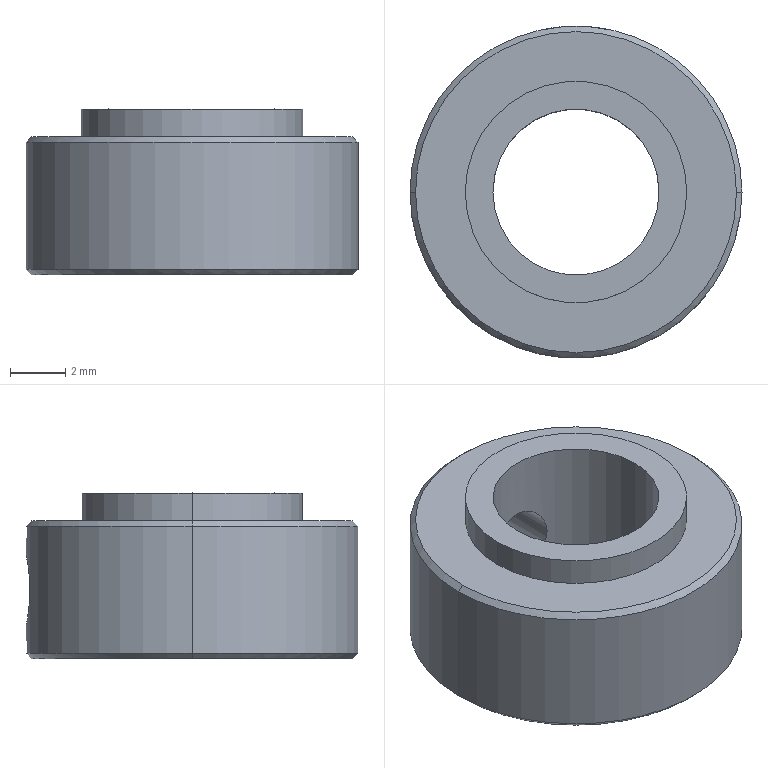Part | SolidWorks | features ICE 2, Chamfer 1, Extrusion 1, HoleWzd 1 | 1 solid | 15 faces | box 12 x 12 x 6 mm | volume 429.723 mm3 | cylinder 8 | cone 4 | plane 3 | commonest cylinder face diameters 2.5 x2 6 x2 8 x2 12 x2
STEP:
#1=CARTESIAN_POINT('',(0.,6.,3.75));
#2=VERTEX_POINT('',#1);
#3=CARTESIAN_POINT('',(0.,6.,1.25));
#4=VERTEX_POINT('',#3);
#5=CARTESIAN_POINT('',(0.,6.,3.75));
#6=CARTESIAN_POINT('',(-0.1634,6.,3.75));
#7=CARTESIAN_POINT('',(-0.3283,5.993,3.717));
#8=CARTESIAN_POINT('',(-0.6292,5.969,3.592));
#9=CARTESIAN_POINT('',(-0.7681,5.952,3.5));
#10=CARTESIAN_POINT('',(-0.9987,5.917,3.269));
#11=CARTESIAN_POINT('',(-1.091,5.9,3.132));
#12=CARTESIAN_POINT('',(-1.217,5.876,2.828));
#13=CARTESIAN_POINT('',(-1.25,5.868,2.666));
#14=CARTESIAN_POINT('',(-1.25,5.868,2.336));
#15=CARTESIAN_POINT('',(-1.217,5.876,2.172));
#16=CARTESIAN_POINT('',(-1.092,5.9,1.87));
#17=CARTESIAN_POINT('',(-0.9992,5.917,1.732));
#18=CARTESIAN_POINT('',(-0.7697,5.952,1.502));
#19=CARTESIAN_POINT('',(-0.6307,5.969,1.409));
#20=CARTESIAN_POINT('',(-0.33,5.993,1.283));
#21=CARTESIAN_POINT('',(-0.1656,6.,1.25));
#22=CARTESIAN_POINT('',(0.,6.,1.25));
#23=B_SPLINE_CURVE_WITH_KNOTS('',3,(#5,#6,#7,#8,#9,#10,#11,#12,#13,#14,#15,#16,#17,#18,#19,#20,#21,#22),.UNSPECIFIED.,.F.,.F.,(4,2,2,2,2,2,2,2,4),(0.003919,0.004409,0.004898,0.005388,0.005878,0.006367,0.006857,0.007347,0.007837),.UNSPECIFIED.);
#24=EDGE_CURVE('',#2,#4,#23,.T.);
#25=ORIENTED_EDGE('',*,*,#24,.F.);
#26=CARTESIAN_POINT('',(0.,3.,3.75));
#27=VERTEX_POINT('',#26);
#28=CARTESIAN_POINT('',(0.,0.,3.75));
#29=DIRECTION('',(0.,-1.,0.));
#30=VECTOR('',#29,1000.);
#31=LINE('',#28,#30);
#32=EDGE_CURVE('',#2,#27,#31,.T.);
#33=ORIENTED_EDGE('',*,*,#32,.T.);
#34=CARTESIAN_POINT('',(0.,3.,1.25));
#35=VERTEX_POINT('',#34);
#36=CARTESIAN_POINT('',(0.,3.,1.25));
#37=CARTESIAN_POINT('',(-0.08362,3.,1.25));
#38=CARTESIAN_POINT('',(-0.1657,2.997,1.258));
#39=CARTESIAN_POINT('',(-0.3268,2.983,1.291));
#40=CARTESIAN_POINT('',(-0.4067,2.973,1.315));
#41=CARTESIAN_POINT('',(-0.6333,2.936,1.41));
#42=CARTESIAN_POINT('',(-0.7706,2.902,1.503));
#43=CARTESIAN_POINT('',(-0.9984,2.832,1.731));
#44=CARTESIAN_POINT('',(-1.091,2.795,1.868));
#45=CARTESIAN_POINT('',(-1.216,2.743,2.168));
#46=CARTESIAN_POINT('',(-1.25,2.727,2.334));
#47=CARTESIAN_POINT('',(-1.25,2.727,2.582));
#48=CARTESIAN_POINT('',(-1.242,2.731,2.666));
#49=CARTESIAN_POINT('',(-1.209,2.746,2.827));
#50=CARTESIAN_POINT('',(-1.185,2.756,2.906));
#51=CARTESIAN_POINT('',(-1.09,2.796,3.134));
#52=CARTESIAN_POINT('',(-0.9979,2.832,3.27));
#53=CARTESIAN_POINT('',(-0.7693,2.902,3.498));
#54=CARTESIAN_POINT('',(-0.6315,2.937,3.591));
#55=CARTESIAN_POINT('',(-0.3311,2.986,3.716));
#56=CARTESIAN_POINT('',(-0.1647,3.,3.75));
#57=CARTESIAN_POINT('',(0.,3.,3.75));
#58=B_SPLINE_CURVE_WITH_KNOTS('',3,(#36,#37,#38,#39,#40,#41,#42,#43,#44,#45,#46,#47,#48,#49,#50,#51,#52,#53,#54,#55,#56,#57),.UNSPECIFIED.,.F.,.F.,(4,2,2,2,2,2,2,2,2,2,4),(0.,0.0002471,0.0004942,0.0009884,0.001483,0.001977,0.002224,0.002471,0.002965,0.003459,0.003954),.UNSPECIFIED.);
#59=EDGE_CURVE('',#35,#27,#58,.T.);
#60=ORIENTED_EDGE('',*,*,#59,.F.);
#61=CARTESIAN_POINT('',(0.,0.,1.25));
#62=DIRECTION('',(0.,-1.,0.));
#63=VECTOR('',#62,1000.);
#64=LINE('',#61,#63);
#65=EDGE_CURVE('',#4,#35,#64,.T.);
#66=ORIENTED_EDGE('',*,*,#65,.F.);
#67=EDGE_LOOP('',(#25,#33,#60,#66));
#68=FACE_OUTER_BOUND('',#67,.T.);
#69=CARTESIAN_POINT('',(0.,0.,2.5));
#70=DIRECTION('',(0.,-1.,0.));
#71=DIRECTION('',(0.,0.,-1.));
#72=AXIS2_PLACEMENT_3D('',#69,#70,#71);
#73=CYLINDRICAL_SURFACE('',#72,1.25);
#74=ADVANCED_FACE('',(#68),#73,.F.);
#75=CARTESIAN_POINT('',(5.8,0.,5.));
#76=VERTEX_POINT('',#75);
#77=CARTESIAN_POINT('',(-5.8,0.,5.));
#78=VERTEX_POINT('',#77);
#79=CARTESIAN_POINT('',(0.,0.,5.));
#80=DIRECTION('',(0.,0.,1.));
#81=DIRECTION('',(1.,0.,0.));
#82=AXIS2_PLACEMENT_3D('',#79,#80,#81);
#83=CIRCLE('',#82,5.8);
#84=EDGE_CURVE('',#76,#78,#83,.T.);
#85=ORIENTED_EDGE('',*,*,#84,.F.);
#86=CARTESIAN_POINT('',(6.,0.,4.8));
#87=VERTEX_POINT('',#86);
#88=CARTESIAN_POINT('',(5.8,0.,5.));
#89=DIRECTION('',(0.7071,0.,-0.7071));
#90=VECTOR('',#89,1000.);
#91=LINE('',#88,#90);
#92=EDGE_CURVE('',#76,#87,#91,.T.);
#93=ORIENTED_EDGE('',*,*,#92,.T.);
#94=CARTESIAN_POINT('',(-6.,0.,4.8));
#95=VERTEX_POINT('',#94);
#96=CARTESIAN_POINT('',(0.,0.,4.8));
#97=DIRECTION('',(0.,0.,-1.));
#98=DIRECTION('',(1.,0.,0.));
#99=AXIS2_PLACEMENT_3D('',#96,#97,#98);
#100=CIRCLE('',#99,6.);
#101=EDGE_CURVE('',#95,#87,#100,.T.);
#102=ORIENTED_EDGE('',*,*,#101,.F.);
#103=CARTESIAN_POINT('',(-5.8,0.,5.));
#104=DIRECTION('',(-0.7071,0.,-0.7071));
#105=VECTOR('',#104,1000.);
#106=LINE('',#103,#105);
#107=EDGE_CURVE('',#78,#95,#106,.T.);
#108=ORIENTED_EDGE('',*,*,#107,.F.);
#109=EDGE_LOOP('',(#85,#93,#102,#108));
#110=FACE_OUTER_BOUND('',#109,.T.);
#111=CARTESIAN_POINT('',(0.,0.,5.));
#112=DIRECTION('',(0.,0.,-1.));
#113=DIRECTION('',(-1.,0.,0.));
#114=AXIS2_PLACEMENT_3D('',#111,#112,#113);
#115=CONICAL_SURFACE('',#114,5.8,0.7854);
#116=ADVANCED_FACE('',(#110),#115,.T.);
#117=CARTESIAN_POINT('',(-5.8,0.,0.));
#118=VERTEX_POINT('',#117);
#119=CARTESIAN_POINT('',(5.8,0.,0.));
#120=VERTEX_POINT('',#119);
#121=CARTESIAN_POINT('',(0.,0.,0.));
#122=DIRECTION('',(0.,0.,-1.));
#123=DIRECTION('',(1.,0.,0.));
#124=AXIS2_PLACEMENT_3D('',#121,#122,#123);
#125=CIRCLE('',#124,5.8);
#126=EDGE_CURVE('',#118,#120,#125,.T.);
#127=ORIENTED_EDGE('',*,*,#126,.F.);
#128=CARTESIAN_POINT('',(-6.,0.,0.2));
#129=VERTEX_POINT('',#128);
#130=CARTESIAN_POINT('',(-6.,0.,0.2));
#131=DIRECTION('',(-0.7071,0.,0.7071));
#132=VECTOR('',#131,1000.);
#133=LINE('',#130,#132);
#134=EDGE_CURVE('',#118,#129,#133,.T.);
#135=ORIENTED_EDGE('',*,*,#134,.T.);
#136=CARTESIAN_POINT('',(6.,0.,0.2));
#137=VERTEX_POINT('',#136);
#138=CARTESIAN_POINT('',(0.,0.,0.2));
#139=DIRECTION('',(0.,0.,1.));
#140=DIRECTION('',(1.,0.,0.));
#141=AXIS2_PLACEMENT_3D('',#138,#139,#140);
#142=CIRCLE('',#141,6.);
#143=EDGE_CURVE('',#137,#129,#142,.T.);
#144=ORIENTED_EDGE('',*,*,#143,.F.);
#145=CARTESIAN_POINT('',(6.,0.,0.2));
#146=DIRECTION('',(0.7071,0.,0.7071));
#147=VECTOR('',#146,1000.);
#148=LINE('',#145,#147);
#149=EDGE_CURVE('',#120,#137,#148,.T.);
#150=ORIENTED_EDGE('',*,*,#149,.F.);
#151=EDGE_LOOP('',(#127,#135,#144,#150));
#152=FACE_OUTER_BOUND('',#151,.T.);
#153=CARTESIAN_POINT('',(0.,0.,0.2));
#154=DIRECTION('',(0.,0.,1.));
#155=DIRECTION('',(1.,0.,0.));
#156=AXIS2_PLACEMENT_3D('',#153,#154,#155);
#157=CONICAL_SURFACE('',#156,6.,0.7854);
#158=ADVANCED_FACE('',(#152),#157,.T.);
#159=CARTESIAN_POINT('',(-3.,0.,0.));
#160=VERTEX_POINT('',#159);
#161=CARTESIAN_POINT('',(3.,0.,0.));
#162=VERTEX_POINT('',#161);
#163=CARTESIAN_POINT('',(0.,0.,0.));
#164=DIRECTION('',(0.,0.,1.));
#165=DIRECTION('',(1.,0.,0.));
#166=AXIS2_PLACEMENT_3D('',#163,#164,#165);
#167=CIRCLE('',#166,3.);
#168=EDGE_CURVE('',#160,#162,#167,.T.);
#169=ORIENTED_EDGE('',*,*,#168,.F.);
#170=CARTESIAN_POINT('',(-3.,0.,6.));
#171=VERTEX_POINT('',#170);
#172=CARTESIAN_POINT('',(-3.,0.,0.));
#173=DIRECTION('',(0.,0.,1.));
#174=VECTOR('',#173,1000.);
#175=LINE('',#172,#174);
#176=EDGE_CURVE('',#160,#171,#175,.T.);
#177=ORIENTED_EDGE('',*,*,#176,.T.);
#178=CARTESIAN_POINT('',(3.,0.,6.));
#179=VERTEX_POINT('',#178);
#180=CARTESIAN_POINT('',(0.,0.,6.));
#181=DIRECTION('',(0.,0.,1.));
#182=DIRECTION('',(1.,0.,0.));
#183=AXIS2_PLACEMENT_3D('',#180,#181,#182);
#184=CIRCLE('',#183,3.);
#185=EDGE_CURVE('',#171,#179,#184,.T.);
#186=ORIENTED_EDGE('',*,*,#185,.T.);
#187=CARTESIAN_POINT('',(3.,0.,0.));
#188=DIRECTION('',(0.,0.,1.));
#189=VECTOR('',#188,1000.);
#190=LINE('',#187,#189);
#191=EDGE_CURVE('',#162,#179,#190,.T.);
#192=ORIENTED_EDGE('',*,*,#191,.F.);
#193=EDGE_LOOP('',(#169,#177,#186,#192));
#194=FACE_OUTER_BOUND('',#193,.T.);
#195=CARTESIAN_POINT('',(0.,0.,0.));
#196=DIRECTION('',(0.,0.,1.));
#197=DIRECTION('',(1.,0.,0.));
#198=AXIS2_PLACEMENT_3D('',#195,#196,#197);
#199=CYLINDRICAL_SURFACE('',#198,3.);
#200=ADVANCED_FACE('',(#194),#199,.F.);
#201=CARTESIAN_POINT('',(4.,0.,6.));
#202=VERTEX_POINT('',#201);
#203=CARTESIAN_POINT('',(-4.,0.,6.));
#204=VERTEX_POINT('',#203);
#205=CARTESIAN_POINT('',(0.,0.,6.));
#206=DIRECTION('',(0.,0.,1.));
#207=DIRECTION('',(1.,0.,0.));
#208=AXIS2_PLACEMENT_3D('',#205,#206,#207);
#209=CIRCLE('',#208,4.);
#210=EDGE_CURVE('',#202,#204,#209,.T.);
#211=ORIENTED_EDGE('',*,*,#210,.F.);
#212=CARTESIAN_POINT('',(4.,0.,5.));
#213=VERTEX_POINT('',#212);
#214=CARTESIAN_POINT('',(4.,0.,6.));
#215=DIRECTION('',(0.,0.,-1.));
#216=VECTOR('',#215,1000.);
#217=LINE('',#214,#216);
#218=EDGE_CURVE('',#202,#213,#217,.T.);
#219=ORIENTED_EDGE('',*,*,#218,.T.);
#220=CARTESIAN_POINT('',(-4.,0.,5.));
#221=VERTEX_POINT('',#220);
#222=CARTESIAN_POINT('',(0.,0.,5.));
#223=DIRECTION('',(0.,0.,1.));
#224=DIRECTION('',(1.,0.,0.));
#225=AXIS2_PLACEMENT_3D('',#222,#223,#224);
#226=CIRCLE('',#225,4.);
#227=EDGE_CURVE('',#213,#221,#226,.T.);
#228=ORIENTED_EDGE('',*,*,#227,.T.);
#229=CARTESIAN_POINT('',(-4.,0.,6.));
#230=DIRECTION('',(0.,0.,-1.));
#231=VECTOR('',#230,1000.);
#232=LINE('',#229,#231);
#233=EDGE_CURVE('',#204,#221,#232,.T.);
#234=ORIENTED_EDGE('',*,*,#233,.F.);
#235=EDGE_LOOP('',(#211,#219,#228,#234));
#236=FACE_OUTER_BOUND('',#235,.T.);
#237=CARTESIAN_POINT('',(0.,0.,6.));
#238=DIRECTION('',(0.,0.,-1.));
#239=DIRECTION('',(-1.,0.,0.));
#240=AXIS2_PLACEMENT_3D('',#237,#238,#239);
#241=CYLINDRICAL_SURFACE('',#240,4.);
#242=ADVANCED_FACE('',(#236),#241,.T.);
#243=CARTESIAN_POINT('',(0.,6.,1.25));
#244=CARTESIAN_POINT('',(0.1657,6.,1.25));
#245=CARTESIAN_POINT('',(0.3282,5.993,1.283));
#246=CARTESIAN_POINT('',(0.6308,5.969,1.408));
#247=CARTESIAN_POINT('',(0.7692,5.952,1.501));
#248=CARTESIAN_POINT('',(0.9991,5.917,1.731));
#249=CARTESIAN_POINT('',(1.092,5.9,1.87));
#250=CARTESIAN_POINT('',(1.217,5.876,2.171));
#251=CARTESIAN_POINT('',(1.25,5.868,2.336));
#252=CARTESIAN_POINT('',(1.25,5.868,2.581));
#253=CARTESIAN_POINT('',(1.242,5.87,2.664));
#254=CARTESIAN_POINT('',(1.21,5.877,2.825));
#255=CARTESIAN_POINT('',(1.186,5.882,2.903));
#256=CARTESIAN_POINT('',(1.092,5.9,3.13));
#257=CARTESIAN_POINT('',(0.9999,5.917,3.268));
#258=CARTESIAN_POINT('',(0.7677,5.952,3.5));
#259=CARTESIAN_POINT('',(0.63,5.969,3.592));
#260=CARTESIAN_POINT('',(0.3278,5.993,3.717));
#261=CARTESIAN_POINT('',(0.1634,6.,3.75));
#262=CARTESIAN_POINT('',(0.,6.,3.75));
#263=B_SPLINE_CURVE_WITH_KNOTS('',3,(#243,#244,#245,#246,#247,#248,#249,#250,#251,#252,#253,#254,#255,#256,#257,#258,#259,#260,#261,#262),.UNSPECIFIED.,.F.,.F.,(4,2,2,2,2,2,2,2,2,4),(0.,0.0004899,0.0009797,0.00147,0.001959,0.002204,0.002449,0.002939,0.003429,0.003919),.UNSPECIFIED.);
#264=EDGE_CURVE('',#4,#2,#263,.T.);
#265=ORIENTED_EDGE('',*,*,#264,.T.);
#266=ORIENTED_EDGE('',*,*,#24,.T.);
#267=EDGE_LOOP('',(#265,#266));
#268=FACE_BOUND('',#267,.T.);
#269=ORIENTED_EDGE('',*,*,#101,.T.);
#270=CARTESIAN_POINT('',(6.,0.,5.));
#271=DIRECTION('',(0.,0.,-1.));
#272=VECTOR('',#271,1000.);
#273=LINE('',#270,#272);
#274=EDGE_CURVE('',#87,#137,#273,.T.);
#275=ORIENTED_EDGE('',*,*,#274,.T.);
#276=ORIENTED_EDGE('',*,*,#143,.T.);
#277=CARTESIAN_POINT('',(-6.,0.,5.));
#278=DIRECTION('',(0.,0.,-1.));
#279=VECTOR('',#278,1000.);
#280=LINE('',#277,#279);
#281=EDGE_CURVE('',#95,#129,#280,.T.);
#282=ORIENTED_EDGE('',*,*,#281,.F.);
#283=EDGE_LOOP('',(#269,#275,#276,#282));
#284=FACE_OUTER_BOUND('',#283,.T.);
#285=CARTESIAN_POINT('',(0.,0.,5.));
#286=DIRECTION('',(0.,0.,-1.));
#287=DIRECTION('',(-1.,0.,0.));
#288=AXIS2_PLACEMENT_3D('',#285,#286,#287);
#289=CYLINDRICAL_SURFACE('',#288,6.);
#290=ADVANCED_FACE('',(#268,#284),#289,.T.);
#291=CARTESIAN_POINT('',(0.,0.,5.));
#292=DIRECTION('',(0.,0.,1.));
#293=DIRECTION('',(1.,0.,0.));
#294=AXIS2_PLACEMENT_3D('',#291,#292,#293);
#295=CIRCLE('',#294,5.8);
#296=EDGE_CURVE('',#78,#76,#295,.T.);
#297=ORIENTED_EDGE('',*,*,#296,.T.);
#298=ORIENTED_EDGE('',*,*,#84,.T.);
#299=EDGE_LOOP('',(#297,#298));
#300=FACE_OUTER_BOUND('',#299,.T.);
#301=CARTESIAN_POINT('',(0.,0.,5.));
#302=DIRECTION('',(0.,0.,1.));
#303=DIRECTION('',(1.,0.,0.));
#304=AXIS2_PLACEMENT_3D('',#301,#302,#303);
#305=CIRCLE('',#304,4.);
#306=EDGE_CURVE('',#221,#213,#305,.T.);
#307=ORIENTED_EDGE('',*,*,#306,.F.);
#308=ORIENTED_EDGE('',*,*,#227,.F.);
#309=EDGE_LOOP('',(#307,#308));
#310=FACE_BOUND('',#309,.T.);
#311=CARTESIAN_POINT('',(0.,0.,5.));
#312=DIRECTION('',(0.,0.,1.));
#313=DIRECTION('',(1.,0.,0.));
#314=AXIS2_PLACEMENT_3D('',#311,#312,#313);
#315=PLANE('',#314);
#316=ADVANCED_FACE('',(#300,#310),#315,.T.);
#317=ORIENTED_EDGE('',*,*,#274,.F.);
#318=CARTESIAN_POINT('',(0.,0.,4.8));
#319=DIRECTION('',(0.,0.,-1.));
#320=DIRECTION('',(1.,0.,0.));
#321=AXIS2_PLACEMENT_3D('',#318,#319,#320);
#322=CIRCLE('',#321,6.);
#323=EDGE_CURVE('',#87,#95,#322,.T.);
#324=ORIENTED_EDGE('',*,*,#323,.T.);
#325=ORIENTED_EDGE('',*,*,#281,.T.);
#326=CARTESIAN_POINT('',(0.,0.,0.2));
#327=DIRECTION('',(0.,0.,1.));
#328=DIRECTION('',(1.,0.,0.));
#329=AXIS2_PLACEMENT_3D('',#326,#327,#328);
#330=CIRCLE('',#329,6.);
#331=EDGE_CURVE('',#129,#137,#330,.T.);
#332=ORIENTED_EDGE('',*,*,#331,.T.);
#333=EDGE_LOOP('',(#317,#324,#325,#332));
#334=FACE_OUTER_BOUND('',#333,.T.);
#335=CARTESIAN_POINT('',(0.,0.,5.));
#336=DIRECTION('',(0.,0.,-1.));
#337=DIRECTION('',(-1.,0.,0.));
#338=AXIS2_PLACEMENT_3D('',#335,#336,#337);
#339=CYLINDRICAL_SURFACE('',#338,6.);
#340=ADVANCED_FACE('',(#334),#339,.T.);
#341=CARTESIAN_POINT('',(0.,0.,0.));
#342=DIRECTION('',(0.,0.,-1.));
#343=DIRECTION('',(1.,0.,0.));
#344=AXIS2_PLACEMENT_3D('',#341,#342,#343);
#345=CIRCLE('',#344,5.8);
#346=EDGE_CURVE('',#120,#118,#345,.T.);
#347=ORIENTED_EDGE('',*,*,#346,.T.);
#348=ORIENTED_EDGE('',*,*,#126,.T.);
#349=EDGE_LOOP('',(#347,#348));
#350=FACE_OUTER_BOUND('',#349,.T.);
#351=CARTESIAN_POINT('',(0.,0.,0.));
#352=DIRECTION('',(0.,0.,1.));
#353=DIRECTION('',(1.,0.,0.));
#354=AXIS2_PLACEMENT_3D('',#351,#352,#353);
#355=CIRCLE('',#354,3.);
#356=EDGE_CURVE('',#162,#160,#355,.T.);
#357=ORIENTED_EDGE('',*,*,#356,.T.);
#358=ORIENTED_EDGE('',*,*,#168,.T.);
#359=EDGE_LOOP('',(#357,#358));
#360=FACE_BOUND('',#359,.T.);
#361=CARTESIAN_POINT('',(0.,0.,0.));
#362=DIRECTION('',(0.,0.,1.));
#363=DIRECTION('',(1.,0.,0.));
#364=AXIS2_PLACEMENT_3D('',#361,#362,#363);
#365=PLANE('',#364);
#366=ADVANCED_FACE('',(#350,#360),#365,.F.);
#367=ORIENTED_EDGE('',*,*,#218,.F.);
#368=CARTESIAN_POINT('',(0.,0.,6.));
#369=DIRECTION('',(0.,0.,1.));
#370=DIRECTION('',(1.,0.,0.));
#371=AXIS2_PLACEMENT_3D('',#368,#369,#370);
#372=CIRCLE('',#371,4.);
#373=EDGE_CURVE('',#204,#202,#372,.T.);
#374=ORIENTED_EDGE('',*,*,#373,.F.);
#375=ORIENTED_EDGE('',*,*,#233,.T.);
#376=ORIENTED_EDGE('',*,*,#306,.T.);
#377=EDGE_LOOP('',(#367,#374,#375,#376));
#378=FACE_OUTER_BOUND('',#377,.T.);
#379=CARTESIAN_POINT('',(0.,0.,6.));
#380=DIRECTION('',(0.,0.,-1.));
#381=DIRECTION('',(-1.,0.,0.));
#382=AXIS2_PLACEMENT_3D('',#379,#380,#381);
#383=CYLINDRICAL_SURFACE('',#382,4.);
#384=ADVANCED_FACE('',(#378),#383,.T.);
#385=CARTESIAN_POINT('',(0.,0.,6.));
#386=DIRECTION('',(0.,0.,1.));
#387=DIRECTION('',(1.,0.,0.));
#388=AXIS2_PLACEMENT_3D('',#385,#386,#387);
#389=CIRCLE('',#388,3.);
#390=EDGE_CURVE('',#179,#171,#389,.T.);
#391=ORIENTED_EDGE('',*,*,#390,.F.);
#392=ORIENTED_EDGE('',*,*,#185,.F.);
#393=EDGE_LOOP('',(#391,#392));
#394=FACE_BOUND('',#393,.T.);
#395=ORIENTED_EDGE('',*,*,#373,.T.);
#396=ORIENTED_EDGE('',*,*,#210,.T.);
#397=EDGE_LOOP('',(#395,#396));
#398=FACE_OUTER_BOUND('',#397,.T.);
#399=CARTESIAN_POINT('',(0.,0.,6.));
#400=DIRECTION('',(0.,0.,1.));
#401=DIRECTION('',(1.,0.,0.));
#402=AXIS2_PLACEMENT_3D('',#399,#400,#401);
#403=PLANE('',#402);
#404=ADVANCED_FACE('',(#394,#398),#403,.T.);
#405=ORIENTED_EDGE('',*,*,#176,.F.);
#406=ORIENTED_EDGE('',*,*,#356,.F.);
#407=ORIENTED_EDGE('',*,*,#191,.T.);
#408=ORIENTED_EDGE('',*,*,#390,.T.);
#409=EDGE_LOOP('',(#405,#406,#407,#408));
#410=FACE_OUTER_BOUND('',#409,.T.);
#411=ORIENTED_EDGE('',*,*,#59,.T.);
#412=CARTESIAN_POINT('',(0.,3.,3.75));
#413=CARTESIAN_POINT('',(0.1646,3.,3.75));
#414=CARTESIAN_POINT('',(0.3304,2.986,3.717));
#415=CARTESIAN_POINT('',(0.6331,2.936,3.59));
#416=CARTESIAN_POINT('',(0.7697,2.902,3.498));
#417=CARTESIAN_POINT('',(0.9421,2.849,3.326));
#418=CARTESIAN_POINT('',(0.9932,2.831,3.263));
#419=CARTESIAN_POINT('',(1.083,2.798,3.129));
#420=CARTESIAN_POINT('',(1.122,2.782,3.056));
#421=CARTESIAN_POINT('',(1.185,2.756,2.906));
#422=CARTESIAN_POINT('',(1.209,2.746,2.828));
#423=CARTESIAN_POINT('',(1.242,2.731,2.667));
#424=CARTESIAN_POINT('',(1.25,2.727,2.583));
#425=CARTESIAN_POINT('',(1.25,2.727,2.336));
#426=CARTESIAN_POINT('',(1.217,2.743,2.17));
#427=CARTESIAN_POINT('',(1.091,2.795,1.868));
#428=CARTESIAN_POINT('',(0.9991,2.831,1.731));
#429=CARTESIAN_POINT('',(0.7697,2.902,1.502));
#430=CARTESIAN_POINT('',(0.6344,2.936,1.41));
#431=CARTESIAN_POINT('',(0.3296,2.986,1.283));
#432=CARTESIAN_POINT('',(0.1671,3.,1.25));
#433=CARTESIAN_POINT('',(0.,3.,1.25));
#434=B_SPLINE_CURVE_WITH_KNOTS('',3,(#412,#413,#414,#415,#416,#417,#418,#419,#420,#421,#422,#423,#424,#425,#426,#427,#428,#429,#430,#431,#432,#433),.UNSPECIFIED.,.F.,.F.,(4,2,2,2,2,2,2,2,2,2,4),(0.003954,0.004448,0.004941,0.005188,0.005435,0.005682,0.005929,0.006423,0.006917,0.00741,0.007904),.UNSPECIFIED.);
#435=EDGE_CURVE('',#27,#35,#434,.T.);
#436=ORIENTED_EDGE('',*,*,#435,.T.);
#437=EDGE_LOOP('',(#411,#436));
#438=FACE_BOUND('',#437,.T.);
#439=CARTESIAN_POINT('',(0.,0.,0.));
#440=DIRECTION('',(0.,0.,1.));
#441=DIRECTION('',(1.,0.,0.));
#442=AXIS2_PLACEMENT_3D('',#439,#440,#441);
#443=CYLINDRICAL_SURFACE('',#442,3.);
#444=ADVANCED_FACE('',(#410,#438),#443,.F.);
#445=ORIENTED_EDGE('',*,*,#134,.F.);
#446=ORIENTED_EDGE('',*,*,#346,.F.);
#447=ORIENTED_EDGE('',*,*,#149,.T.);
#448=ORIENTED_EDGE('',*,*,#331,.F.);
#449=EDGE_LOOP('',(#445,#446,#447,#448));
#450=FACE_OUTER_BOUND('',#449,.T.);
#451=CARTESIAN_POINT('',(0.,0.,0.2));
#452=DIRECTION('',(0.,0.,1.));
#453=DIRECTION('',(1.,0.,0.));
#454=AXIS2_PLACEMENT_3D('',#451,#452,#453);
#455=CONICAL_SURFACE('',#454,6.,0.7854);
#456=ADVANCED_FACE('',(#450),#455,.T.);
#457=ORIENTED_EDGE('',*,*,#92,.F.);
#458=ORIENTED_EDGE('',*,*,#296,.F.);
#459=ORIENTED_EDGE('',*,*,#107,.T.);
#460=ORIENTED_EDGE('',*,*,#323,.F.);
#461=EDGE_LOOP('',(#457,#458,#459,#460));
#462=FACE_OUTER_BOUND('',#461,.T.);
#463=CARTESIAN_POINT('',(0.,0.,5.));
#464=DIRECTION('',(0.,0.,-1.));
#465=DIRECTION('',(-1.,0.,0.));
#466=AXIS2_PLACEMENT_3D('',#463,#464,#465);
#467=CONICAL_SURFACE('',#466,5.8,0.7854);
#468=ADVANCED_FACE('',(#462),#467,.T.);
#469=ORIENTED_EDGE('',*,*,#32,.F.);
#470=ORIENTED_EDGE('',*,*,#264,.F.);
#471=ORIENTED_EDGE('',*,*,#65,.T.);
#472=ORIENTED_EDGE('',*,*,#435,.F.);
#473=EDGE_LOOP('',(#469,#470,#471,#472));
#474=FACE_OUTER_BOUND('',#473,.T.);
#475=CARTESIAN_POINT('',(0.,0.,2.5));
#476=DIRECTION('',(0.,-1.,0.));
#477=DIRECTION('',(0.,0.,-1.));
#478=AXIS2_PLACEMENT_3D('',#475,#476,#477);
#479=CYLINDRICAL_SURFACE('',#478,1.25);
#480=ADVANCED_FACE('',(#474),#479,.F.);
#481=CLOSED_SHELL('',(#74,#116,#158,#200,#242,#290,#316,#340,#366,#384,#404,#444,#456,#468,#480));
#482=MANIFOLD_SOLID_BREP('',#481);
#483=CARTESIAN_POINT('',(0.,0.,0.));
#484=DIRECTION('',(0.,0.,1.));
#485=DIRECTION('',(1.,0.,0.));
#486=AXIS2_PLACEMENT_3D('',#483,#484,#485);
#487=(LENGTH_UNIT()NAMED_UNIT(*)SI_UNIT(.MILLI.,.METRE.));
#488=UNCERTAINTY_MEASURE_WITH_UNIT(LENGTH_MEASURE(0.00001),#487,'','');
#489=(NAMED_UNIT(*)PLANE_ANGLE_UNIT()SI_UNIT($,.RADIAN.));
#490=(NAMED_UNIT(*)SI_UNIT($,.STERADIAN.)SOLID_ANGLE_UNIT());
#491=(GEOMETRIC_REPRESENTATION_CONTEXT(3)GLOBAL_UNCERTAINTY_ASSIGNED_CONTEXT((#488))GLOBAL_UNIT_ASSIGNED_CONTEXT((#487,#489,#490))REPRESENTATION_CONTEXT('',''));
#492=ADVANCED_BREP_SHAPE_REPRESENTATION('',(#482,#486),#491);